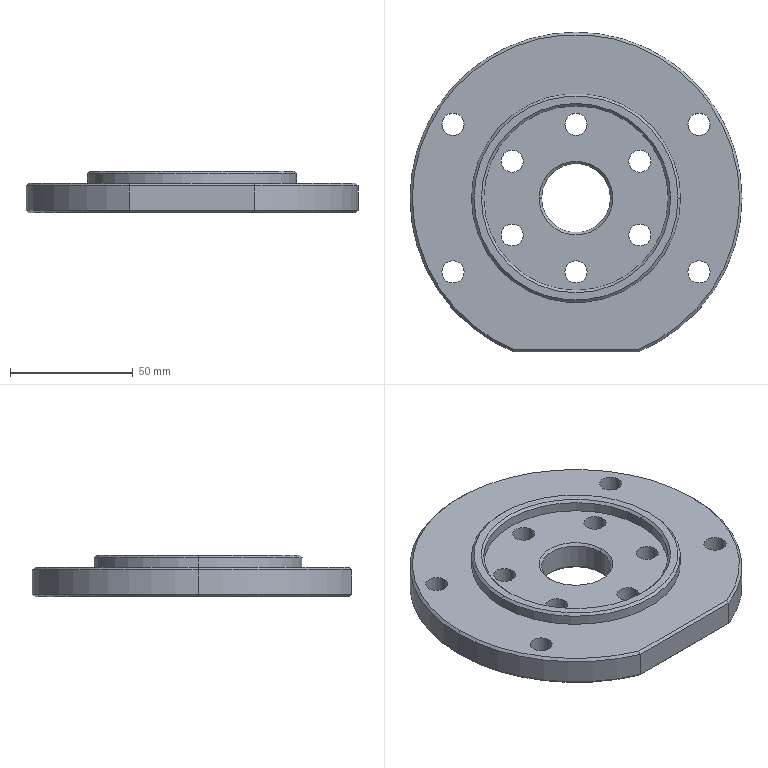Part | STEP file | YCD14007A-08.03.08.02 Adapter Flange (Cylinder) | 1 solid | 50 faces | box 135 x 130 x 17 mm | volume 160209 mm3 | cylinder 29 | cone 14 | plane 7 | commonest cylinder face diameters 9 x20 135 x3 28 x2 75 x2 85 x2